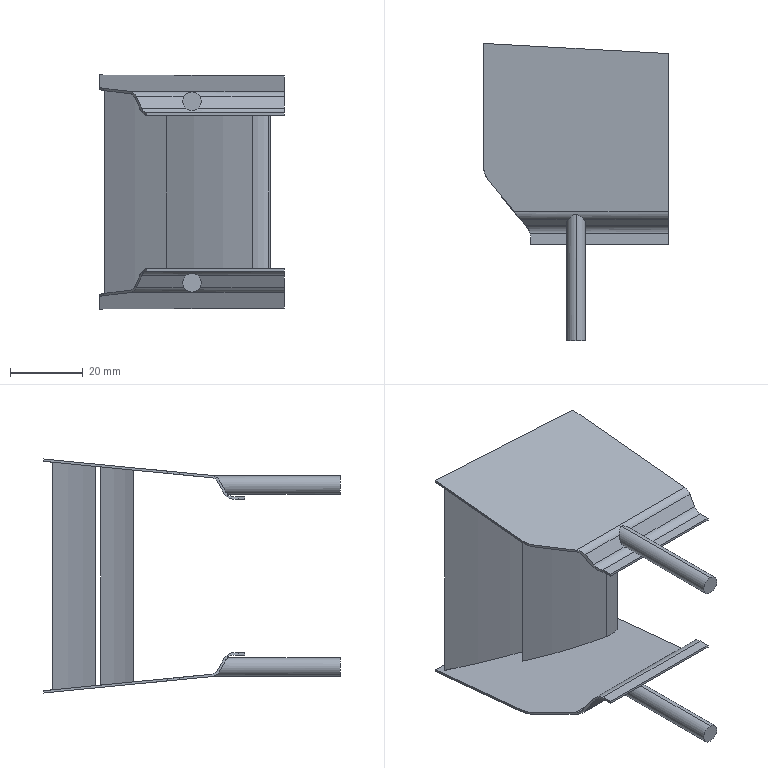Part | SolidWorks | features ICE 4, Extrusion 1, MirrorSolid 1 | 1 solid | 54 faces | box 50.8 x 81.634 x 64.383 mm | volume 11608 mm3 | plane 29 | cylinder 25 | commonest cylinder face diameters 5.08 x8 10.16 x4 3.81 x2 6.35 x2 0.84 x1 4.595 x1